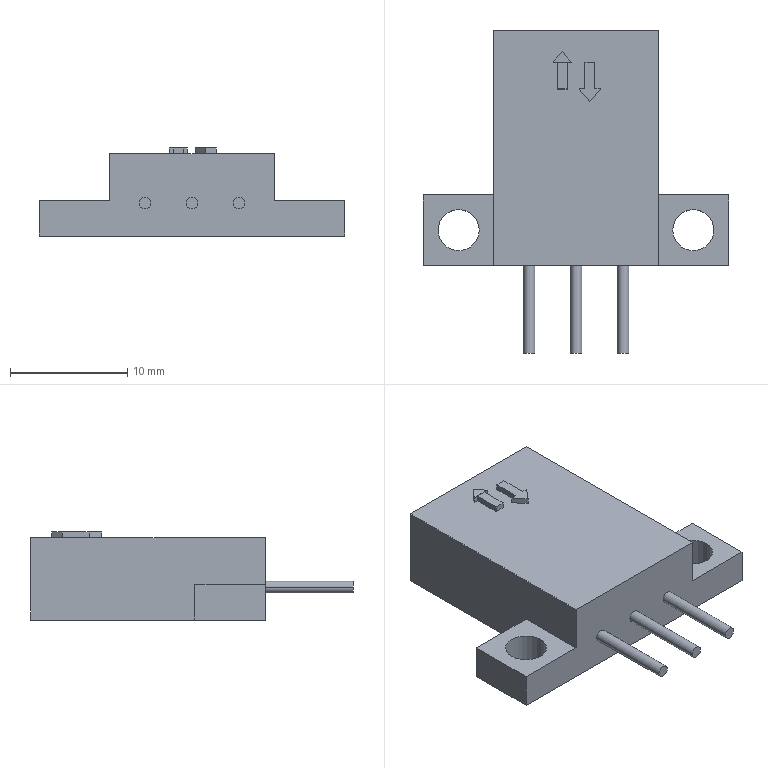Part | NX | features BREP 1 | 1 solid | 47 faces | box 26 x 27.5 x 7.5 mm | volume 2123 mm3 | plane 37 | cylinder 10 | commonest cylinder face diameters 1 x6 3.5 x4
STEP:
#1=CARTESIAN_POINT('',(4.,19.5,5.5));
#2=VERTEX_POINT('',#1);
#3=CARTESIAN_POINT('',(4.,19.5,1.5));
#4=VERTEX_POINT('',#3);
#5=CARTESIAN_POINT('',(4.,19.5,5.5));
#6=DIRECTION('',(0.,0.,-1.));
#7=VECTOR('',#6,1000.);
#8=LINE('',#5,#7);
#9=EDGE_CURVE('',#2,#4,#8,.T.);
#10=ORIENTED_EDGE('',*,*,#9,.T.);
#11=CARTESIAN_POINT('',(-4.,19.5,1.5));
#12=VERTEX_POINT('',#11);
#13=CARTESIAN_POINT('',(-4.,19.5,1.5));
#14=DIRECTION('',(-1.,0.,0.));
#15=VECTOR('',#14,1000.);
#16=LINE('',#13,#15);
#17=EDGE_CURVE('',#4,#12,#16,.T.);
#18=ORIENTED_EDGE('',*,*,#17,.T.);
#19=CARTESIAN_POINT('',(-4.,19.5,5.5));
#20=VERTEX_POINT('',#19);
#21=CARTESIAN_POINT('',(-4.,19.5,5.5));
#22=DIRECTION('',(0.,0.,1.));
#23=VECTOR('',#22,1000.);
#24=LINE('',#21,#23);
#25=EDGE_CURVE('',#12,#20,#24,.T.);
#26=ORIENTED_EDGE('',*,*,#25,.T.);
#27=CARTESIAN_POINT('',(-4.,19.5,5.5));
#28=DIRECTION('',(1.,0.,0.));
#29=VECTOR('',#28,1000.);
#30=LINE('',#27,#29);
#31=EDGE_CURVE('',#20,#2,#30,.T.);
#32=ORIENTED_EDGE('',*,*,#31,.T.);
#33=EDGE_LOOP('',(#10,#18,#26,#32));
#34=FACE_BOUND('',#33,.T.);
#35=CARTESIAN_POINT('',(0.,19.5,0.));
#36=DIRECTION('',(0.,-1.,0.));
#37=DIRECTION('',(0.,0.,-1.));
#38=AXIS2_PLACEMENT_3D('',#35,#36,#37);
#39=PLANE('',#38);
#40=ADVANCED_FACE('',(#34),#39,.F.);
#41=CARTESIAN_POINT('',(4.,20.,1.5));
#42=VERTEX_POINT('',#41);
#43=CARTESIAN_POINT('',(-4.,20.,1.5));
#44=VERTEX_POINT('',#43);
#45=CARTESIAN_POINT('',(-4.,20.,1.5));
#46=DIRECTION('',(-1.,0.,0.));
#47=VECTOR('',#46,1000.);
#48=LINE('',#45,#47);
#49=EDGE_CURVE('',#42,#44,#48,.T.);
#50=ORIENTED_EDGE('',*,*,#49,.T.);
#51=CARTESIAN_POINT('',(-4.,19.5,1.5));
#52=DIRECTION('',(0.,1.,0.));
#53=VECTOR('',#52,1000.);
#54=LINE('',#51,#53);
#55=EDGE_CURVE('',#12,#44,#54,.T.);
#56=ORIENTED_EDGE('',*,*,#55,.F.);
#57=ORIENTED_EDGE('',*,*,#17,.F.);
#58=CARTESIAN_POINT('',(4.,19.5,1.5));
#59=DIRECTION('',(0.,1.,0.));
#60=VECTOR('',#59,1000.);
#61=LINE('',#58,#60);
#62=EDGE_CURVE('',#4,#42,#61,.T.);
#63=ORIENTED_EDGE('',*,*,#62,.T.);
#64=EDGE_LOOP('',(#50,#56,#57,#63));
#65=FACE_BOUND('',#64,.T.);
#66=CARTESIAN_POINT('',(-4.,19.5,1.5));
#67=DIRECTION('',(0.,0.,-1.));
#68=DIRECTION('',(-1.,0.,0.));
#69=AXIS2_PLACEMENT_3D('',#66,#67,#68);
#70=PLANE('',#69);
#71=ADVANCED_FACE('',(#65),#70,.F.);
#72=CARTESIAN_POINT('',(-4.,20.,5.5));
#73=VERTEX_POINT('',#72);
#74=CARTESIAN_POINT('',(-4.,20.,5.5));
#75=DIRECTION('',(0.,0.,1.));
#76=VECTOR('',#75,1000.);
#77=LINE('',#74,#76);
#78=EDGE_CURVE('',#44,#73,#77,.T.);
#79=ORIENTED_EDGE('',*,*,#78,.T.);
#80=CARTESIAN_POINT('',(-4.,19.5,5.5));
#81=DIRECTION('',(0.,1.,0.));
#82=VECTOR('',#81,1000.);
#83=LINE('',#80,#82);
#84=EDGE_CURVE('',#20,#73,#83,.T.);
#85=ORIENTED_EDGE('',*,*,#84,.F.);
#86=ORIENTED_EDGE('',*,*,#25,.F.);
#87=ORIENTED_EDGE('',*,*,#55,.T.);
#88=EDGE_LOOP('',(#79,#85,#86,#87));
#89=FACE_BOUND('',#88,.T.);
#90=CARTESIAN_POINT('',(-4.,19.5,5.5));
#91=DIRECTION('',(-1.,0.,0.));
#92=DIRECTION('',(0.,0.,1.));
#93=AXIS2_PLACEMENT_3D('',#90,#91,#92);
#94=PLANE('',#93);
#95=ADVANCED_FACE('',(#89),#94,.F.);
#96=CARTESIAN_POINT('',(4.,20.,5.5));
#97=VERTEX_POINT('',#96);
#98=CARTESIAN_POINT('',(-4.,20.,5.5));
#99=DIRECTION('',(1.,0.,0.));
#100=VECTOR('',#99,1000.);
#101=LINE('',#98,#100);
#102=EDGE_CURVE('',#73,#97,#101,.T.);
#103=ORIENTED_EDGE('',*,*,#102,.T.);
#104=CARTESIAN_POINT('',(4.,19.5,5.5));
#105=DIRECTION('',(0.,1.,0.));
#106=VECTOR('',#105,1000.);
#107=LINE('',#104,#106);
#108=EDGE_CURVE('',#2,#97,#107,.T.);
#109=ORIENTED_EDGE('',*,*,#108,.F.);
#110=ORIENTED_EDGE('',*,*,#31,.F.);
#111=ORIENTED_EDGE('',*,*,#84,.T.);
#112=EDGE_LOOP('',(#103,#109,#110,#111));
#113=FACE_BOUND('',#112,.T.);
#114=CARTESIAN_POINT('',(-4.,19.5,5.5));
#115=DIRECTION('',(0.,0.,1.));
#116=DIRECTION('',(1.,0.,0.));
#117=AXIS2_PLACEMENT_3D('',#114,#115,#116);
#118=PLANE('',#117);
#119=ADVANCED_FACE('',(#113),#118,.F.);
#120=CARTESIAN_POINT('',(4.,20.,5.5));
#121=DIRECTION('',(0.,0.,-1.));
#122=VECTOR('',#121,1000.);
#123=LINE('',#120,#122);
#124=EDGE_CURVE('',#97,#42,#123,.T.);
#125=ORIENTED_EDGE('',*,*,#124,.T.);
#126=ORIENTED_EDGE('',*,*,#62,.F.);
#127=ORIENTED_EDGE('',*,*,#9,.F.);
#128=ORIENTED_EDGE('',*,*,#108,.T.);
#129=EDGE_LOOP('',(#125,#126,#127,#128));
#130=FACE_BOUND('',#129,.T.);
#131=CARTESIAN_POINT('',(4.,19.5,5.5));
#132=DIRECTION('',(1.,0.,0.));
#133=DIRECTION('',(0.,0.,-1.));
#134=AXIS2_PLACEMENT_3D('',#131,#132,#133);
#135=PLANE('',#134);
#136=ADVANCED_FACE('',(#130),#135,.F.);
#137=CARTESIAN_POINT('',(3.5,-7.5,2.8));
#138=VERTEX_POINT('',#137);
#139=CARTESIAN_POINT('',(4.5,-7.5,2.8));
#140=VERTEX_POINT('',#139);
#141=CARTESIAN_POINT('',(4.,-7.5,2.8));
#142=DIRECTION('',(0.,-1.,0.));
#143=DIRECTION('',(1.,0.,0.));
#144=AXIS2_PLACEMENT_3D('',#141,#142,#143);
#145=CIRCLE('',#144,0.5);
#146=EDGE_CURVE('',#138,#140,#145,.T.);
#147=ORIENTED_EDGE('',*,*,#146,.T.);
#148=CARTESIAN_POINT('',(4.,-7.5,2.8));
#149=DIRECTION('',(0.,-1.,0.));
#150=DIRECTION('',(1.,0.,0.));
#151=AXIS2_PLACEMENT_3D('',#148,#149,#150);
#152=CIRCLE('',#151,0.5);
#153=EDGE_CURVE('',#140,#138,#152,.T.);
#154=ORIENTED_EDGE('',*,*,#153,.T.);
#155=EDGE_LOOP('',(#147,#154));
#156=FACE_BOUND('',#155,.T.);
#157=CARTESIAN_POINT('',(4.,-7.5,2.8));
#158=DIRECTION('',(0.,-1.,0.));
#159=DIRECTION('',(1.,0.,0.));
#160=AXIS2_PLACEMENT_3D('',#157,#158,#159);
#161=PLANE('',#160);
#162=ADVANCED_FACE('',(#156),#161,.T.);
#163=CARTESIAN_POINT('',(4.5,0.,2.8));
#164=VERTEX_POINT('',#163);
#165=CARTESIAN_POINT('',(4.5,-7.5,2.8));
#166=DIRECTION('',(0.,1.,0.));
#167=VECTOR('',#166,1000.);
#168=LINE('',#165,#167);
#169=EDGE_CURVE('',#140,#164,#168,.T.);
#170=ORIENTED_EDGE('',*,*,#169,.F.);
#171=ORIENTED_EDGE('',*,*,#146,.F.);
#172=CARTESIAN_POINT('',(3.5,0.,2.8));
#173=VERTEX_POINT('',#172);
#174=CARTESIAN_POINT('',(3.5,-7.5,2.8));
#175=DIRECTION('',(0.,1.,0.));
#176=VECTOR('',#175,1000.);
#177=LINE('',#174,#176);
#178=EDGE_CURVE('',#138,#173,#177,.T.);
#179=ORIENTED_EDGE('',*,*,#178,.T.);
#180=CARTESIAN_POINT('',(4.,0.,2.8));
#181=DIRECTION('',(0.,-1.,0.));
#182=DIRECTION('',(-1.,0.,0.));
#183=AXIS2_PLACEMENT_3D('',#180,#181,#182);
#184=CIRCLE('',#183,0.5);
#185=EDGE_CURVE('',#173,#164,#184,.T.);
#186=ORIENTED_EDGE('',*,*,#185,.T.);
#187=EDGE_LOOP('',(#170,#171,#179,#186));
#188=FACE_BOUND('',#187,.T.);
#189=CARTESIAN_POINT('',(4.,-7.5,2.8));
#190=DIRECTION('',(0.,1.,0.));
#191=DIRECTION('',(-1.,0.,0.));
#192=AXIS2_PLACEMENT_3D('',#189,#190,#191);
#193=CYLINDRICAL_SURFACE('',#192,0.5);
#194=ADVANCED_FACE('',(#188),#193,.T.);
#195=CARTESIAN_POINT('',(-0.5,-7.5,2.8));
#196=VERTEX_POINT('',#195);
#197=CARTESIAN_POINT('',(0.5,-7.5,2.8));
#198=VERTEX_POINT('',#197);
#199=CARTESIAN_POINT('',(0.,-7.5,2.8));
#200=DIRECTION('',(0.,-1.,0.));
#201=DIRECTION('',(1.,0.,0.));
#202=AXIS2_PLACEMENT_3D('',#199,#200,#201);
#203=CIRCLE('',#202,0.5);
#204=EDGE_CURVE('',#196,#198,#203,.T.);
#205=ORIENTED_EDGE('',*,*,#204,.T.);
#206=CARTESIAN_POINT('',(0.,-7.5,2.8));
#207=DIRECTION('',(0.,-1.,0.));
#208=DIRECTION('',(1.,0.,0.));
#209=AXIS2_PLACEMENT_3D('',#206,#207,#208);
#210=CIRCLE('',#209,0.5);
#211=EDGE_CURVE('',#198,#196,#210,.T.);
#212=ORIENTED_EDGE('',*,*,#211,.T.);
#213=EDGE_LOOP('',(#205,#212));
#214=FACE_BOUND('',#213,.T.);
#215=CARTESIAN_POINT('',(0.,-7.5,2.8));
#216=DIRECTION('',(0.,-1.,0.));
#217=DIRECTION('',(1.,0.,0.));
#218=AXIS2_PLACEMENT_3D('',#215,#216,#217);
#219=PLANE('',#218);
#220=ADVANCED_FACE('',(#214),#219,.T.);
#221=CARTESIAN_POINT('',(0.5,0.,2.8));
#222=VERTEX_POINT('',#221);
#223=CARTESIAN_POINT('',(0.5,-7.5,2.8));
#224=DIRECTION('',(0.,1.,0.));
#225=VECTOR('',#224,1000.);
#226=LINE('',#223,#225);
#227=EDGE_CURVE('',#198,#222,#226,.T.);
#228=ORIENTED_EDGE('',*,*,#227,.F.);
#229=ORIENTED_EDGE('',*,*,#204,.F.);
#230=CARTESIAN_POINT('',(-0.5,0.,2.8));
#231=VERTEX_POINT('',#230);
#232=CARTESIAN_POINT('',(-0.5,-7.5,2.8));
#233=DIRECTION('',(0.,1.,0.));
#234=VECTOR('',#233,1000.);
#235=LINE('',#232,#234);
#236=EDGE_CURVE('',#196,#231,#235,.T.);
#237=ORIENTED_EDGE('',*,*,#236,.T.);
#238=CARTESIAN_POINT('',(0.,0.,2.8));
#239=DIRECTION('',(0.,-1.,0.));
#240=DIRECTION('',(-1.,0.,0.));
#241=AXIS2_PLACEMENT_3D('',#238,#239,#240);
#242=CIRCLE('',#241,0.5);
#243=EDGE_CURVE('',#231,#222,#242,.T.);
#244=ORIENTED_EDGE('',*,*,#243,.T.);
#245=EDGE_LOOP('',(#228,#229,#237,#244));
#246=FACE_BOUND('',#245,.T.);
#247=CARTESIAN_POINT('',(0.,-7.5,2.8));
#248=DIRECTION('',(0.,1.,0.));
#249=DIRECTION('',(-1.,0.,0.));
#250=AXIS2_PLACEMENT_3D('',#247,#248,#249);
#251=CYLINDRICAL_SURFACE('',#250,0.5);
#252=ADVANCED_FACE('',(#246),#251,.T.);
#253=CARTESIAN_POINT('',(-4.5,-7.5,2.8));
#254=VERTEX_POINT('',#253);
#255=CARTESIAN_POINT('',(-3.5,-7.5,2.8));
#256=VERTEX_POINT('',#255);
#257=CARTESIAN_POINT('',(-4.,-7.5,2.8));
#258=DIRECTION('',(0.,-1.,0.));
#259=DIRECTION('',(1.,0.,0.));
#260=AXIS2_PLACEMENT_3D('',#257,#258,#259);
#261=CIRCLE('',#260,0.5);
#262=EDGE_CURVE('',#254,#256,#261,.T.);
#263=ORIENTED_EDGE('',*,*,#262,.T.);
#264=CARTESIAN_POINT('',(-4.,-7.5,2.8));
#265=DIRECTION('',(0.,-1.,0.));
#266=DIRECTION('',(1.,0.,0.));
#267=AXIS2_PLACEMENT_3D('',#264,#265,#266);
#268=CIRCLE('',#267,0.5);
#269=EDGE_CURVE('',#256,#254,#268,.T.);
#270=ORIENTED_EDGE('',*,*,#269,.T.);
#271=EDGE_LOOP('',(#263,#270));
#272=FACE_BOUND('',#271,.T.);
#273=CARTESIAN_POINT('',(-4.,-7.5,2.8));
#274=DIRECTION('',(0.,-1.,0.));
#275=DIRECTION('',(1.,0.,0.));
#276=AXIS2_PLACEMENT_3D('',#273,#274,#275);
#277=PLANE('',#276);
#278=ADVANCED_FACE('',(#272),#277,.T.);
#279=CARTESIAN_POINT('',(-3.5,0.,2.8));
#280=VERTEX_POINT('',#279);
#281=CARTESIAN_POINT('',(-3.5,-7.5,2.8));
#282=DIRECTION('',(0.,1.,0.));
#283=VECTOR('',#282,1000.);
#284=LINE('',#281,#283);
#285=EDGE_CURVE('',#256,#280,#284,.T.);
#286=ORIENTED_EDGE('',*,*,#285,.F.);
#287=ORIENTED_EDGE('',*,*,#262,.F.);
#288=CARTESIAN_POINT('',(-4.5,0.,2.8));
#289=VERTEX_POINT('',#288);
#290=CARTESIAN_POINT('',(-4.5,-7.5,2.8));
#291=DIRECTION('',(0.,1.,0.));
#292=VECTOR('',#291,1000.);
#293=LINE('',#290,#292);
#294=EDGE_CURVE('',#254,#289,#293,.T.);
#295=ORIENTED_EDGE('',*,*,#294,.T.);
#296=CARTESIAN_POINT('',(-4.,0.,2.8));
#297=DIRECTION('',(0.,-1.,0.));
#298=DIRECTION('',(-1.,0.,0.));
#299=AXIS2_PLACEMENT_3D('',#296,#297,#298);
#300=CIRCLE('',#299,0.5);
#301=EDGE_CURVE('',#289,#280,#300,.T.);
#302=ORIENTED_EDGE('',*,*,#301,.T.);
#303=EDGE_LOOP('',(#286,#287,#295,#302));
#304=FACE_BOUND('',#303,.T.);
#305=CARTESIAN_POINT('',(-4.,-7.5,2.8));
#306=DIRECTION('',(0.,1.,0.));
#307=DIRECTION('',(-1.,0.,0.));
#308=AXIS2_PLACEMENT_3D('',#305,#306,#307);
#309=CYLINDRICAL_SURFACE('',#308,0.5);
#310=ADVANCED_FACE('',(#304),#309,.T.);
#311=CARTESIAN_POINT('',(-11.75,3.,3.));
#312=VERTEX_POINT('',#311);
#313=CARTESIAN_POINT('',(-11.75,3.,0.));
#314=VERTEX_POINT('',#313);
#315=CARTESIAN_POINT('',(-11.75,3.,3.));
#316=DIRECTION('',(0.,0.,1.));
#317=VECTOR('',#316,1000.);
#318=LINE('',#315,#317);
#319=EDGE_CURVE('',#312,#314,#318,.F.);
#320=ORIENTED_EDGE('',*,*,#319,.T.);
#321=CARTESIAN_POINT('',(-8.25,3.,0.));
#322=VERTEX_POINT('',#321);
#323=CARTESIAN_POINT('',(-10.,3.,0.));
#324=DIRECTION('',(0.,0.,1.));
#325=DIRECTION('',(1.,0.,0.));
#326=AXIS2_PLACEMENT_3D('',#323,#324,#325);
#327=CIRCLE('',#326,1.75);
#328=EDGE_CURVE('',#322,#314,#327,.T.);
#329=ORIENTED_EDGE('',*,*,#328,.F.);
#330=CARTESIAN_POINT('',(-8.25,3.,3.));
#331=VERTEX_POINT('',#330);
#332=CARTESIAN_POINT('',(-8.25,3.,3.));
#333=DIRECTION('',(0.,0.,1.));
#334=VECTOR('',#333,1000.);
#335=LINE('',#332,#334);
#336=EDGE_CURVE('',#331,#322,#335,.F.);
#337=ORIENTED_EDGE('',*,*,#336,.F.);
#338=CARTESIAN_POINT('',(-10.,3.,3.));
#339=DIRECTION('',(0.,0.,1.));
#340=DIRECTION('',(1.,0.,0.));
#341=AXIS2_PLACEMENT_3D('',#338,#339,#340);
#342=CIRCLE('',#341,1.75);
#343=EDGE_CURVE('',#331,#312,#342,.T.);
#344=ORIENTED_EDGE('',*,*,#343,.T.);
#345=EDGE_LOOP('',(#320,#329,#337,#344));
#346=FACE_BOUND('',#345,.T.);
#347=CARTESIAN_POINT('',(-10.,3.,3.));
#348=DIRECTION('',(0.,0.,1.));
#349=DIRECTION('',(1.,0.,0.));
#350=AXIS2_PLACEMENT_3D('',#347,#348,#349);
#351=CYLINDRICAL_SURFACE('',#350,1.75);
#352=ADVANCED_FACE('',(#346),#351,.F.);
#353=CARTESIAN_POINT('',(8.25,3.,3.));
#354=VERTEX_POINT('',#353);
#355=CARTESIAN_POINT('',(8.25,3.,0.));
#356=VERTEX_POINT('',#355);
#357=CARTESIAN_POINT('',(8.25,3.,3.));
#358=DIRECTION('',(0.,0.,1.));
#359=VECTOR('',#358,1000.);
#360=LINE('',#357,#359);
#361=EDGE_CURVE('',#354,#356,#360,.F.);
#362=ORIENTED_EDGE('',*,*,#361,.T.);
#363=CARTESIAN_POINT('',(11.75,3.,0.));
#364=VERTEX_POINT('',#363);
#365=CARTESIAN_POINT('',(10.,3.,0.));
#366=DIRECTION('',(0.,0.,1.));
#367=DIRECTION('',(1.,0.,0.));
#368=AXIS2_PLACEMENT_3D('',#365,#366,#367);
#369=CIRCLE('',#368,1.75);
#370=EDGE_CURVE('',#364,#356,#369,.T.);
#371=ORIENTED_EDGE('',*,*,#370,.F.);
#372=CARTESIAN_POINT('',(11.75,3.,3.));
#373=VERTEX_POINT('',#372);
#374=CARTESIAN_POINT('',(11.75,3.,3.));
#375=DIRECTION('',(0.,0.,1.));
#376=VECTOR('',#375,1000.);
#377=LINE('',#374,#376);
#378=EDGE_CURVE('',#373,#364,#377,.F.);
#379=ORIENTED_EDGE('',*,*,#378,.F.);
#380=CARTESIAN_POINT('',(10.,3.,3.));
#381=DIRECTION('',(0.,0.,1.));
#382=DIRECTION('',(1.,0.,0.));
#383=AXIS2_PLACEMENT_3D('',#380,#381,#382);
#384=CIRCLE('',#383,1.75);
#385=EDGE_CURVE('',#373,#354,#384,.T.);
#386=ORIENTED_EDGE('',*,*,#385,.T.);
#387=EDGE_LOOP('',(#362,#371,#379,#386));
#388=FACE_BOUND('',#387,.T.);
#389=CARTESIAN_POINT('',(10.,3.,3.));
#390=DIRECTION('',(0.,0.,1.));
#391=DIRECTION('',(1.,0.,0.));
#392=AXIS2_PLACEMENT_3D('',#389,#390,#391);
#393=CYLINDRICAL_SURFACE('',#392,1.75);
#394=ADVANCED_FACE('',(#388),#393,.F.);
#395=CARTESIAN_POINT('',(1.592,17.295,7.5));
#396=VERTEX_POINT('',#395);
#397=CARTESIAN_POINT('',(1.592,15.02,7.5));
#398=VERTEX_POINT('',#397);
#399=CARTESIAN_POINT('',(1.592,0.,7.5));
#400=DIRECTION('',(0.,-1.,0.));
#401=VECTOR('',#400,1000.);
#402=LINE('',#399,#401);
#403=EDGE_CURVE('',#396,#398,#402,.T.);
#404=ORIENTED_EDGE('',*,*,#403,.F.);
#405=CARTESIAN_POINT('',(0.7557,17.295,7.5));
#406=VERTEX_POINT('',#405);
#407=CARTESIAN_POINT('',(0.,17.295,7.5));
#408=DIRECTION('',(1.,0.,0.));
#409=VECTOR('',#408,1000.);
#410=LINE('',#407,#409);
#411=EDGE_CURVE('',#406,#396,#410,.T.);
#412=ORIENTED_EDGE('',*,*,#411,.F.);
#413=CARTESIAN_POINT('',(0.7557,15.02,7.5));
#414=VERTEX_POINT('',#413);
#415=CARTESIAN_POINT('',(0.7557,0.,7.5));
#416=DIRECTION('',(0.,-1.,0.));
#417=VECTOR('',#416,1000.);
#418=LINE('',#415,#417);
#419=EDGE_CURVE('',#406,#414,#418,.T.);
#420=ORIENTED_EDGE('',*,*,#419,.T.);
#421=CARTESIAN_POINT('',(0.2749,15.02,7.5));
#422=VERTEX_POINT('',#421);
#423=CARTESIAN_POINT('',(0.,15.02,7.5));
#424=DIRECTION('',(1.,0.,0.));
#425=VECTOR('',#424,1000.);
#426=LINE('',#423,#425);
#427=EDGE_CURVE('',#422,#414,#426,.T.);
#428=ORIENTED_EDGE('',*,*,#427,.F.);
#429=CARTESIAN_POINT('',(1.174,13.95,7.5));
#430=VERTEX_POINT('',#429);
#431=CARTESIAN_POINT('',(7.559,6.351,7.5));
#432=DIRECTION('',(-0.6433,0.7656,0.));
#433=VECTOR('',#432,1000.);
#434=LINE('',#431,#433);
#435=EDGE_CURVE('',#430,#422,#434,.T.);
#436=ORIENTED_EDGE('',*,*,#435,.F.);
#437=CARTESIAN_POINT('',(2.073,15.02,7.5));
#438=VERTEX_POINT('',#437);
#439=CARTESIAN_POINT('',(-6.183,5.195,7.5));
#440=DIRECTION('',(-0.6433,-0.7656,0.));
#441=VECTOR('',#440,1000.);
#442=LINE('',#439,#441);
#443=EDGE_CURVE('',#438,#430,#442,.T.);
#444=ORIENTED_EDGE('',*,*,#443,.F.);
#445=CARTESIAN_POINT('',(0.,15.02,7.5));
#446=DIRECTION('',(1.,0.,0.));
#447=VECTOR('',#446,1000.);
#448=LINE('',#445,#447);
#449=EDGE_CURVE('',#398,#438,#448,.T.);
#450=ORIENTED_EDGE('',*,*,#449,.F.);
#451=EDGE_LOOP('',(#404,#412,#420,#428,#436,#444,#450));
#452=FACE_BOUND('',#451,.T.);
#453=CARTESIAN_POINT('',(0.,0.,7.5));
#454=DIRECTION('',(0.,0.,1.));
#455=DIRECTION('',(1.,0.,0.));
#456=AXIS2_PLACEMENT_3D('',#453,#454,#455);
#457=PLANE('',#456);
#458=ADVANCED_FACE('',(#452),#457,.T.);
#459=CARTESIAN_POINT('',(1.592,15.02,7.));
#460=VERTEX_POINT('',#459);
#461=CARTESIAN_POINT('',(2.073,15.02,7.));
#462=VERTEX_POINT('',#461);
#463=CARTESIAN_POINT('',(0.,15.02,7.));
#464=DIRECTION('',(1.,0.,0.));
#465=VECTOR('',#464,1000.);
#466=LINE('',#463,#465);
#467=EDGE_CURVE('',#460,#462,#466,.T.);
#468=ORIENTED_EDGE('',*,*,#467,.F.);
#469=CARTESIAN_POINT('',(1.592,15.02,7.5));
#470=DIRECTION('',(0.,0.,-1.));
#471=VECTOR('',#470,1000.);
#472=LINE('',#469,#471);
#473=EDGE_CURVE('',#398,#460,#472,.T.);
#474=ORIENTED_EDGE('',*,*,#473,.F.);
#475=ORIENTED_EDGE('',*,*,#449,.T.);
#476=CARTESIAN_POINT('',(2.073,15.02,7.5));
#477=DIRECTION('',(0.,0.,-1.));
#478=VECTOR('',#477,1000.);
#479=LINE('',#476,#478);
#480=EDGE_CURVE('',#438,#462,#479,.T.);
#481=ORIENTED_EDGE('',*,*,#480,.T.);
#482=EDGE_LOOP('',(#468,#474,#475,#481));
#483=FACE_BOUND('',#482,.T.);
#484=CARTESIAN_POINT('',(0.,15.02,7.5));
#485=DIRECTION('',(0.,1.,0.));
#486=DIRECTION('',(0.,0.,1.));
#487=AXIS2_PLACEMENT_3D('',#484,#485,#486);
#488=PLANE('',#487);
#489=ADVANCED_FACE('',(#483),#488,.T.);
#490=CARTESIAN_POINT('',(1.174,13.95,7.));
#491=VERTEX_POINT('',#490);
#492=CARTESIAN_POINT('',(-6.183,5.195,7.));
#493=DIRECTION('',(-0.6433,-0.7656,0.));
#494=VECTOR('',#493,1000.);
#495=LINE('',#492,#494);
#496=EDGE_CURVE('',#462,#491,#495,.T.);
#497=ORIENTED_EDGE('',*,*,#496,.F.);
#498=ORIENTED_EDGE('',*,*,#480,.F.);
#499=ORIENTED_EDGE('',*,*,#443,.T.);
#500=CARTESIAN_POINT('',(1.174,13.95,7.5));
#501=DIRECTION('',(0.,0.,-1.));
#502=VECTOR('',#501,1000.);
#503=LINE('',#500,#502);
#504=EDGE_CURVE('',#430,#491,#503,.T.);
#505=ORIENTED_EDGE('',*,*,#504,.T.);
#506=EDGE_LOOP('',(#497,#498,#499,#505));
#507=FACE_BOUND('',#506,.T.);
#508=CARTESIAN_POINT('',(-6.183,5.195,7.5));
#509=DIRECTION('',(0.7656,-0.6433,0.));
#510=DIRECTION('',(0.6433,0.7656,0.));
#511=AXIS2_PLACEMENT_3D('',#508,#509,#510);
#512=PLANE('',#511);
#513=ADVANCED_FACE('',(#507),#512,.T.);
#514=CARTESIAN_POINT('',(0.2749,15.02,7.));
#515=VERTEX_POINT('',#514);
#516=CARTESIAN_POINT('',(7.559,6.351,7.));
#517=DIRECTION('',(-0.6433,0.7656,0.));
#518=VECTOR('',#517,1000.);
#519=LINE('',#516,#518);
#520=EDGE_CURVE('',#491,#515,#519,.T.);
#521=ORIENTED_EDGE('',*,*,#520,.F.);
#522=ORIENTED_EDGE('',*,*,#504,.F.);
#523=ORIENTED_EDGE('',*,*,#435,.T.);
#524=CARTESIAN_POINT('',(0.2749,15.02,7.5));
#525=DIRECTION('',(0.,0.,-1.));
#526=VECTOR('',#525,1000.);
#527=LINE('',#524,#526);
#528=EDGE_CURVE('',#422,#515,#527,.T.);
#529=ORIENTED_EDGE('',*,*,#528,.T.);
#530=EDGE_LOOP('',(#521,#522,#523,#529));
#531=FACE_BOUND('',#530,.T.);
#532=CARTESIAN_POINT('',(7.559,6.351,7.5));
#533=DIRECTION('',(-0.7656,-0.6433,0.));
#534=DIRECTION('',(0.6433,-0.7656,0.));
#535=AXIS2_PLACEMENT_3D('',#532,#533,#534);
#536=PLANE('',#535);
#537=ADVANCED_FACE('',(#531),#536,.T.);
#538=CARTESIAN_POINT('',(0.7557,15.02,7.));
#539=VERTEX_POINT('',#538);
#540=CARTESIAN_POINT('',(0.,15.02,7.));
#541=DIRECTION('',(1.,0.,0.));
#542=VECTOR('',#541,1000.);
#543=LINE('',#540,#542);
#544=EDGE_CURVE('',#515,#539,#543,.T.);
#545=ORIENTED_EDGE('',*,*,#544,.F.);
#546=ORIENTED_EDGE('',*,*,#528,.F.);
#547=ORIENTED_EDGE('',*,*,#427,.T.);
#548=CARTESIAN_POINT('',(0.7557,15.02,7.5));
#549=DIRECTION('',(0.,0.,-1.));
#550=VECTOR('',#549,1000.);
#551=LINE('',#548,#550);
#552=EDGE_CURVE('',#414,#539,#551,.T.);
#553=ORIENTED_EDGE('',*,*,#552,.T.);
#554=EDGE_LOOP('',(#545,#546,#547,#553));
#555=FACE_BOUND('',#554,.T.);
#556=CARTESIAN_POINT('',(0.,15.02,7.5));
#557=DIRECTION('',(0.,1.,0.));
#558=DIRECTION('',(0.,0.,1.));
#559=AXIS2_PLACEMENT_3D('',#556,#557,#558);
#560=PLANE('',#559);
#561=ADVANCED_FACE('',(#555),#560,.T.);
#562=CARTESIAN_POINT('',(0.7557,17.295,7.));
#563=VERTEX_POINT('',#562);
#564=CARTESIAN_POINT('',(0.7557,0.,7.));
#565=DIRECTION('',(0.,-1.,0.));
#566=VECTOR('',#565,1000.);
#567=LINE('',#564,#566);
#568=EDGE_CURVE('',#563,#539,#567,.T.);
#569=ORIENTED_EDGE('',*,*,#568,.T.);
#570=ORIENTED_EDGE('',*,*,#552,.F.);
#571=ORIENTED_EDGE('',*,*,#419,.F.);
#572=CARTESIAN_POINT('',(0.7557,17.295,7.5));
#573=DIRECTION('',(0.,0.,-1.));
#574=VECTOR('',#573,1000.);
#575=LINE('',#572,#574);
#576=EDGE_CURVE('',#406,#563,#575,.T.);
#577=ORIENTED_EDGE('',*,*,#576,.T.);
#578=EDGE_LOOP('',(#569,#570,#571,#577));
#579=FACE_BOUND('',#578,.T.);
#580=CARTESIAN_POINT('',(0.7557,0.,7.5));
#581=DIRECTION('',(1.,0.,0.));
#582=DIRECTION('',(0.,1.,0.));
#583=AXIS2_PLACEMENT_3D('',#580,#581,#582);
#584=PLANE('',#583);
#585=ADVANCED_FACE('',(#579),#584,.F.);
#586=CARTESIAN_POINT('',(1.592,17.295,7.));
#587=VERTEX_POINT('',#586);
#588=CARTESIAN_POINT('',(0.,17.295,7.));
#589=DIRECTION('',(1.,0.,0.));
#590=VECTOR('',#589,1000.);
#591=LINE('',#588,#590);
#592=EDGE_CURVE('',#563,#587,#591,.T.);
#593=ORIENTED_EDGE('',*,*,#592,.F.);
#594=ORIENTED_EDGE('',*,*,#576,.F.);
#595=ORIENTED_EDGE('',*,*,#411,.T.);
#596=CARTESIAN_POINT('',(1.592,17.295,7.5));
#597=DIRECTION('',(0.,0.,-1.));
#598=VECTOR('',#597,1000.);
#599=LINE('',#596,#598);
#600=EDGE_CURVE('',#396,#587,#599,.T.);
#601=ORIENTED_EDGE('',*,*,#600,.T.);
#602=EDGE_LOOP('',(#593,#594,#595,#601));
#603=FACE_BOUND('',#602,.T.);
#604=CARTESIAN_POINT('',(0.,17.295,7.5));
#605=DIRECTION('',(0.,1.,0.));
#606=DIRECTION('',(-1.,0.,0.));
#607=AXIS2_PLACEMENT_3D('',#604,#605,#606);
#608=PLANE('',#607);
#609=ADVANCED_FACE('',(#603),#608,.T.);
#610=CARTESIAN_POINT('',(1.592,0.,7.));
#611=DIRECTION('',(0.,-1.,0.));
#612=VECTOR('',#611,1000.);
#613=LINE('',#610,#612);
#614=EDGE_CURVE('',#587,#460,#613,.T.);
#615=ORIENTED_EDGE('',*,*,#614,.F.);
#616=ORIENTED_EDGE('',*,*,#600,.F.);
#617=ORIENTED_EDGE('',*,*,#403,.T.);
#618=ORIENTED_EDGE('',*,*,#473,.T.);
#619=EDGE_LOOP('',(#615,#616,#617,#618));
#620=FACE_BOUND('',#619,.T.);
#621=CARTESIAN_POINT('',(1.592,0.,7.5));
#622=DIRECTION('',(1.,0.,0.));
#623=DIRECTION('',(0.,0.,-1.));
#624=AXIS2_PLACEMENT_3D('',#621,#622,#623);
#625=PLANE('',#624);
#626=ADVANCED_FACE('',(#620),#625,.T.);
#627=CARTESIAN_POINT('',(-1.592,15.02,7.5));
#628=VERTEX_POINT('',#627);
#629=CARTESIAN_POINT('',(-0.7557,15.02,7.5));
#630=VERTEX_POINT('',#629);
#631=CARTESIAN_POINT('',(0.,15.02,7.5));
#632=DIRECTION('',(1.,0.,0.));
#633=VECTOR('',#632,1000.);
#634=LINE('',#631,#633);
#635=EDGE_CURVE('',#628,#630,#634,.T.);
#636=ORIENTED_EDGE('',*,*,#635,.T.);
#637=CARTESIAN_POINT('',(-0.7557,17.295,7.5));
#638=VERTEX_POINT('',#637);
#639=CARTESIAN_POINT('',(-0.7557,0.,7.5));
#640=DIRECTION('',(0.,1.,0.));
#641=VECTOR('',#640,1000.);
#642=LINE('',#639,#641);
#643=EDGE_CURVE('',#630,#638,#642,.T.);
#644=ORIENTED_EDGE('',*,*,#643,.T.);
#645=CARTESIAN_POINT('',(-1.592,17.295,7.5));
#646=VERTEX_POINT('',#645);
#647=CARTESIAN_POINT('',(0.,17.295,7.5));
#648=DIRECTION('',(1.,0.,0.));
#649=VECTOR('',#648,1000.);
#650=LINE('',#647,#649);
#651=EDGE_CURVE('',#646,#638,#650,.T.);
#652=ORIENTED_EDGE('',*,*,#651,.F.);
#653=CARTESIAN_POINT('',(-1.592,0.,7.5));
#654=DIRECTION('',(0.,1.,0.));
#655=VECTOR('',#654,1000.);
#656=LINE('',#653,#655);
#657=EDGE_CURVE('',#628,#646,#656,.T.);
#658=ORIENTED_EDGE('',*,*,#657,.F.);
#659=EDGE_LOOP('',(#636,#644,#652,#658));
#660=FACE_BOUND('',#659,.T.);
#661=CARTESIAN_POINT('',(0.,0.,7.5));
#662=DIRECTION('',(0.,0.,1.));
#663=DIRECTION('',(1.,0.,0.));
#664=AXIS2_PLACEMENT_3D('',#661,#662,#663);
#665=PLANE('',#664);
#666=ADVANCED_FACE('',(#660),#665,.T.);
#667=CARTESIAN_POINT('',(-1.592,15.02,7.));
#668=VERTEX_POINT('',#667);
#669=CARTESIAN_POINT('',(-1.592,17.295,7.));
#670=VERTEX_POINT('',#669);
#671=CARTESIAN_POINT('',(-1.592,0.,7.));
#672=DIRECTION('',(0.,1.,0.));
#673=VECTOR('',#672,1000.);
#674=LINE('',#671,#673);
#675=EDGE_CURVE('',#668,#670,#674,.T.);
#676=ORIENTED_EDGE('',*,*,#675,.F.);
#677=CARTESIAN_POINT('',(-1.592,15.02,7.5));
#678=DIRECTION('',(0.,0.,-1.));
#679=VECTOR('',#678,1000.);
#680=LINE('',#677,#679);
#681=EDGE_CURVE('',#628,#668,#680,.T.);
#682=ORIENTED_EDGE('',*,*,#681,.F.);
#683=ORIENTED_EDGE('',*,*,#657,.T.);
#684=CARTESIAN_POINT('',(-1.592,17.295,7.5));
#685=DIRECTION('',(0.,0.,-1.));
#686=VECTOR('',#685,1000.);
#687=LINE('',#684,#686);
#688=EDGE_CURVE('',#646,#670,#687,.T.);
#689=ORIENTED_EDGE('',*,*,#688,.T.);
#690=EDGE_LOOP('',(#676,#682,#683,#689));
#691=FACE_BOUND('',#690,.T.);
#692=CARTESIAN_POINT('',(-1.592,0.,7.5));
#693=DIRECTION('',(-1.,0.,0.));
#694=DIRECTION('',(0.,0.,1.));
#695=AXIS2_PLACEMENT_3D('',#692,#693,#694);
#696=PLANE('',#695);
#697=ADVANCED_FACE('',(#691),#696,.T.);
#698=CARTESIAN_POINT('',(-0.7557,17.295,7.));
#699=VERTEX_POINT('',#698);
#700=CARTESIAN_POINT('',(0.,17.295,7.));
#701=DIRECTION('',(1.,0.,0.));
#702=VECTOR('',#701,1000.);
#703=LINE('',#700,#702);
#704=EDGE_CURVE('',#670,#699,#703,.T.);
#705=ORIENTED_EDGE('',*,*,#704,.F.);
#706=ORIENTED_EDGE('',*,*,#688,.F.);
#707=ORIENTED_EDGE('',*,*,#651,.T.);
#708=CARTESIAN_POINT('',(-0.7557,17.295,7.5));
#709=DIRECTION('',(0.,0.,-1.));
#710=VECTOR('',#709,1000.);
#711=LINE('',#708,#710);
#712=EDGE_CURVE('',#638,#699,#711,.T.);
#713=ORIENTED_EDGE('',*,*,#712,.T.);
#714=EDGE_LOOP('',(#705,#706,#707,#713));
#715=FACE_BOUND('',#714,.T.);
#716=CARTESIAN_POINT('',(0.,17.295,7.5));
#717=DIRECTION('',(0.,1.,0.));
#718=DIRECTION('',(0.,0.,1.));
#719=AXIS2_PLACEMENT_3D('',#716,#717,#718);
#720=PLANE('',#719);
#721=ADVANCED_FACE('',(#715),#720,.T.);
#722=CARTESIAN_POINT('',(-0.7557,15.02,7.));
#723=VERTEX_POINT('',#722);
#724=CARTESIAN_POINT('',(-0.7557,0.,7.));
#725=DIRECTION('',(0.,1.,0.));
#726=VECTOR('',#725,1000.);
#727=LINE('',#724,#726);
#728=EDGE_CURVE('',#723,#699,#727,.T.);
#729=ORIENTED_EDGE('',*,*,#728,.T.);
#730=ORIENTED_EDGE('',*,*,#712,.F.);
#731=ORIENTED_EDGE('',*,*,#643,.F.);
#732=CARTESIAN_POINT('',(-0.7557,15.02,7.5));
#733=DIRECTION('',(0.,0.,-1.));
#734=VECTOR('',#733,1000.);
#735=LINE('',#732,#734);
#736=EDGE_CURVE('',#630,#723,#735,.T.);
#737=ORIENTED_EDGE('',*,*,#736,.T.);
#738=EDGE_LOOP('',(#729,#730,#731,#737));
#739=FACE_BOUND('',#738,.T.);
#740=CARTESIAN_POINT('',(-0.7557,0.,7.5));
#741=DIRECTION('',(-1.,0.,0.));
#742=DIRECTION('',(0.,-1.,0.));
#743=AXIS2_PLACEMENT_3D('',#740,#741,#742);
#744=PLANE('',#743);
#745=ADVANCED_FACE('',(#739),#744,.F.);
#746=CARTESIAN_POINT('',(0.,15.02,7.));
#747=DIRECTION('',(1.,0.,0.));
#748=VECTOR('',#747,1000.);
#749=LINE('',#746,#748);
#750=EDGE_CURVE('',#668,#723,#749,.T.);
#751=ORIENTED_EDGE('',*,*,#750,.T.);
#752=ORIENTED_EDGE('',*,*,#736,.F.);
#753=ORIENTED_EDGE('',*,*,#635,.F.);
#754=ORIENTED_EDGE('',*,*,#681,.T.);
#755=EDGE_LOOP('',(#751,#752,#753,#754));
#756=FACE_BOUND('',#755,.T.);
#757=CARTESIAN_POINT('',(0.,15.02,7.5));
#758=DIRECTION('',(0.,1.,0.));
#759=DIRECTION('',(0.,0.,1.));
#760=AXIS2_PLACEMENT_3D('',#757,#758,#759);
#761=PLANE('',#760);
#762=ADVANCED_FACE('',(#756),#761,.F.);
#763=CARTESIAN_POINT('',(-0.3905,17.301,7.5));
#764=VERTEX_POINT('',#763);
#765=CARTESIAN_POINT('',(-1.957,17.301,7.5));
#766=VERTEX_POINT('',#765);
#767=CARTESIAN_POINT('',(0.,17.301,7.5));
#768=DIRECTION('',(-1.,0.,0.));
#769=VECTOR('',#768,1000.);
#770=LINE('',#767,#769);
#771=EDGE_CURVE('',#764,#766,#770,.T.);
#772=ORIENTED_EDGE('',*,*,#771,.F.);
#773=CARTESIAN_POINT('',(-1.174,18.21,7.5));
#774=VERTEX_POINT('',#773);
#775=CARTESIAN_POINT('',(8.333,7.186,7.5));
#776=DIRECTION('',(0.6531,-0.7573,0.));
#777=VECTOR('',#776,1000.);
#778=LINE('',#775,#777);
#779=EDGE_CURVE('',#774,#764,#778,.T.);
#780=ORIENTED_EDGE('',*,*,#779,.F.);
#781=CARTESIAN_POINT('',(-9.679,8.347,7.5));
#782=DIRECTION('',(0.6531,0.7573,0.));
#783=VECTOR('',#782,1000.);
#784=LINE('',#781,#783);
#785=EDGE_CURVE('',#766,#774,#784,.T.);
#786=ORIENTED_EDGE('',*,*,#785,.F.);
#787=EDGE_LOOP('',(#772,#780,#786));
#788=FACE_BOUND('',#787,.T.);
#789=CARTESIAN_POINT('',(0.,0.,7.5));
#790=DIRECTION('',(0.,0.,1.));
#791=DIRECTION('',(1.,0.,0.));
#792=AXIS2_PLACEMENT_3D('',#789,#790,#791);
#793=PLANE('',#792);
#794=ADVANCED_FACE('',(#788),#793,.T.);
#795=CARTESIAN_POINT('',(-1.957,17.301,7.));
#796=VERTEX_POINT('',#795);
#797=CARTESIAN_POINT('',(-1.174,18.21,7.));
#798=VERTEX_POINT('',#797);
#799=CARTESIAN_POINT('',(-9.679,8.347,7.));
#800=DIRECTION('',(0.6531,0.7573,0.));
#801=VECTOR('',#800,1000.);
#802=LINE('',#799,#801);
#803=EDGE_CURVE('',#796,#798,#802,.T.);
#804=ORIENTED_EDGE('',*,*,#803,.F.);
#805=CARTESIAN_POINT('',(-1.957,17.301,7.5));
#806=DIRECTION('',(0.,0.,-1.));
#807=VECTOR('',#806,1000.);
#808=LINE('',#805,#807);
#809=EDGE_CURVE('',#766,#796,#808,.T.);
#810=ORIENTED_EDGE('',*,*,#809,.F.);
#811=ORIENTED_EDGE('',*,*,#785,.T.);
#812=CARTESIAN_POINT('',(-1.174,18.21,7.5));
#813=DIRECTION('',(0.,0.,-1.));
#814=VECTOR('',#813,1000.);
#815=LINE('',#812,#814);
#816=EDGE_CURVE('',#774,#798,#815,.T.);
#817=ORIENTED_EDGE('',*,*,#816,.T.);
#818=EDGE_LOOP('',(#804,#810,#811,#817));
#819=FACE_BOUND('',#818,.T.);
#820=CARTESIAN_POINT('',(-9.679,8.347,7.5));
#821=DIRECTION('',(-0.7573,0.6531,0.));
#822=DIRECTION('',(-0.6531,-0.7573,0.));
#823=AXIS2_PLACEMENT_3D('',#820,#821,#822);
#824=PLANE('',#823);
#825=ADVANCED_FACE('',(#819),#824,.T.);
#826=CARTESIAN_POINT('',(-0.3905,17.301,7.));
#827=VERTEX_POINT('',#826);
#828=CARTESIAN_POINT('',(8.333,7.186,7.));
#829=DIRECTION('',(0.6531,-0.7573,0.));
#830=VECTOR('',#829,1000.);
#831=LINE('',#828,#830);
#832=EDGE_CURVE('',#798,#827,#831,.T.);
#833=ORIENTED_EDGE('',*,*,#832,.F.);
#834=ORIENTED_EDGE('',*,*,#816,.F.);
#835=ORIENTED_EDGE('',*,*,#779,.T.);
#836=CARTESIAN_POINT('',(-0.3905,17.301,7.5));
#837=DIRECTION('',(0.,0.,-1.));
#838=VECTOR('',#837,1000.);
#839=LINE('',#836,#838);
#840=EDGE_CURVE('',#764,#827,#839,.T.);
#841=ORIENTED_EDGE('',*,*,#840,.T.);
#842=EDGE_LOOP('',(#833,#834,#835,#841));
#843=FACE_BOUND('',#842,.T.);
#844=CARTESIAN_POINT('',(8.333,7.186,7.5));
#845=DIRECTION('',(0.7573,0.6531,0.));
#846=DIRECTION('',(-0.6531,0.7573,0.));
#847=AXIS2_PLACEMENT_3D('',#844,#845,#846);
#848=PLANE('',#847);
#849=ADVANCED_FACE('',(#843),#848,.T.);
#850=CARTESIAN_POINT('',(0.,17.301,7.));
#851=DIRECTION('',(-1.,0.,0.));
#852=VECTOR('',#851,1000.);
#853=LINE('',#850,#852);
#854=EDGE_CURVE('',#827,#796,#853,.T.);
#855=ORIENTED_EDGE('',*,*,#854,.F.);
#856=ORIENTED_EDGE('',*,*,#840,.F.);
#857=ORIENTED_EDGE('',*,*,#771,.T.);
#858=ORIENTED_EDGE('',*,*,#809,.T.);
#859=EDGE_LOOP('',(#855,#856,#857,#858));
#860=FACE_BOUND('',#859,.T.);
#861=CARTESIAN_POINT('',(0.,17.301,7.5));
#862=DIRECTION('',(0.,-1.,0.));
#863=DIRECTION('',(0.,0.,-1.));
#864=AXIS2_PLACEMENT_3D('',#861,#862,#863);
#865=PLANE('',#864);
#866=ADVANCED_FACE('',(#860),#865,.T.);
#867=CARTESIAN_POINT('',(13.,6.,3.));
#868=VERTEX_POINT('',#867);
#869=CARTESIAN_POINT('',(13.,0.,3.));
#870=VERTEX_POINT('',#869);
#871=CARTESIAN_POINT('',(13.,6.,3.));
#872=DIRECTION('',(0.,-1.,0.));
#873=VECTOR('',#872,1000.);
#874=LINE('',#871,#873);
#875=EDGE_CURVE('',#868,#870,#874,.T.);
#876=ORIENTED_EDGE('',*,*,#875,.F.);
#877=CARTESIAN_POINT('',(7.,6.,3.));
#878=VERTEX_POINT('',#877);
#879=CARTESIAN_POINT('',(13.,6.,3.));
#880=DIRECTION('',(1.,0.,0.));
#881=VECTOR('',#880,1000.);
#882=LINE('',#879,#881);
#883=EDGE_CURVE('',#878,#868,#882,.T.);
#884=ORIENTED_EDGE('',*,*,#883,.F.);
#885=CARTESIAN_POINT('',(7.,0.,3.));
#886=VERTEX_POINT('',#885);
#887=CARTESIAN_POINT('',(7.,6.,3.));
#888=DIRECTION('',(0.,1.,0.));
#889=VECTOR('',#888,1000.);
#890=LINE('',#887,#889);
#891=EDGE_CURVE('',#886,#878,#890,.T.);
#892=ORIENTED_EDGE('',*,*,#891,.F.);
#893=CARTESIAN_POINT('',(13.,0.,3.));
#894=DIRECTION('',(-1.,0.,0.));
#895=VECTOR('',#894,1000.);
#896=LINE('',#893,#895);
#897=EDGE_CURVE('',#870,#886,#896,.T.);
#898=ORIENTED_EDGE('',*,*,#897,.F.);
#899=EDGE_LOOP('',(#876,#884,#892,#898));
#900=FACE_BOUND('',#899,.T.);
#901=ORIENTED_EDGE('',*,*,#385,.F.);
#902=CARTESIAN_POINT('',(10.,3.,3.));
#903=DIRECTION('',(0.,0.,1.));
#904=DIRECTION('',(1.,0.,0.));
#905=AXIS2_PLACEMENT_3D('',#902,#903,#904);
#906=CIRCLE('',#905,1.75);
#907=EDGE_CURVE('',#354,#373,#906,.T.);
#908=ORIENTED_EDGE('',*,*,#907,.F.);
#909=EDGE_LOOP('',(#901,#908));
#910=FACE_BOUND('',#909,.T.);
#911=CARTESIAN_POINT('',(0.,0.,3.));
#912=DIRECTION('',(0.,0.,1.));
#913=DIRECTION('',(1.,0.,0.));
#914=AXIS2_PLACEMENT_3D('',#911,#912,#913);
#915=PLANE('',#914);
#916=ADVANCED_FACE('',(#900,#910),#915,.T.);
#917=CARTESIAN_POINT('',(-13.,0.,3.));
#918=VERTEX_POINT('',#917);
#919=CARTESIAN_POINT('',(-13.,6.,3.));
#920=VERTEX_POINT('',#919);
#921=CARTESIAN_POINT('',(-13.,6.,3.));
#922=DIRECTION('',(0.,1.,0.));
#923=VECTOR('',#922,1000.);
#924=LINE('',#921,#923);
#925=EDGE_CURVE('',#918,#920,#924,.T.);
#926=ORIENTED_EDGE('',*,*,#925,.F.);
#927=CARTESIAN_POINT('',(-7.,0.,3.));
#928=VERTEX_POINT('',#927);
#929=CARTESIAN_POINT('',(-13.,0.,3.));
#930=DIRECTION('',(-1.,0.,0.));
#931=VECTOR('',#930,1000.);
#932=LINE('',#929,#931);
#933=EDGE_CURVE('',#928,#918,#932,.T.);
#934=ORIENTED_EDGE('',*,*,#933,.F.);
#935=CARTESIAN_POINT('',(-7.,6.,3.));
#936=VERTEX_POINT('',#935);
#937=CARTESIAN_POINT('',(-7.,6.,3.));
#938=DIRECTION('',(0.,-1.,0.));
#939=VECTOR('',#938,1000.);
#940=LINE('',#937,#939);
#941=EDGE_CURVE('',#936,#928,#940,.T.);
#942=ORIENTED_EDGE('',*,*,#941,.F.);
#943=CARTESIAN_POINT('',(-13.,6.,3.));
#944=DIRECTION('',(1.,0.,0.));
#945=VECTOR('',#944,1000.);
#946=LINE('',#943,#945);
#947=EDGE_CURVE('',#920,#936,#946,.T.);
#948=ORIENTED_EDGE('',*,*,#947,.F.);
#949=EDGE_LOOP('',(#926,#934,#942,#948));
#950=FACE_BOUND('',#949,.T.);
#951=ORIENTED_EDGE('',*,*,#343,.F.);
#952=CARTESIAN_POINT('',(-10.,3.,3.));
#953=DIRECTION('',(0.,0.,1.));
#954=DIRECTION('',(1.,0.,0.));
#955=AXIS2_PLACEMENT_3D('',#952,#953,#954);
#956=CIRCLE('',#955,1.75);
#957=EDGE_CURVE('',#312,#331,#956,.T.);
#958=ORIENTED_EDGE('',*,*,#957,.F.);
#959=EDGE_LOOP('',(#951,#958));
#960=FACE_BOUND('',#959,.T.);
#961=CARTESIAN_POINT('',(0.,0.,3.));
#962=DIRECTION('',(0.,0.,1.));
#963=DIRECTION('',(1.,0.,0.));
#964=AXIS2_PLACEMENT_3D('',#961,#962,#963);
#965=PLANE('',#964);
#966=ADVANCED_FACE('',(#950,#960),#965,.T.);
#967=CARTESIAN_POINT('',(-7.,20.,0.));
#968=VERTEX_POINT('',#967);
#969=CARTESIAN_POINT('',(-7.,6.,0.));
#970=VERTEX_POINT('',#969);
#971=CARTESIAN_POINT('',(-7.,0.,0.));
#972=DIRECTION('',(0.,-1.,0.));
#973=VECTOR('',#972,1000.);
#974=LINE('',#971,#973);
#975=EDGE_CURVE('',#968,#970,#974,.T.);
#976=ORIENTED_EDGE('',*,*,#975,.F.);
#977=CARTESIAN_POINT('',(7.,20.,0.));
#978=VERTEX_POINT('',#977);
#979=CARTESIAN_POINT('',(0.,20.,0.));
#980=DIRECTION('',(1.,0.,0.));
#981=VECTOR('',#980,1000.);
#982=LINE('',#979,#981);
#983=EDGE_CURVE('',#968,#978,#982,.T.);
#984=ORIENTED_EDGE('',*,*,#983,.T.);
#985=CARTESIAN_POINT('',(7.,6.,0.));
#986=VERTEX_POINT('',#985);
#987=CARTESIAN_POINT('',(7.,0.,0.));
#988=DIRECTION('',(0.,-1.,0.));
#989=VECTOR('',#988,1000.);
#990=LINE('',#987,#989);
#991=EDGE_CURVE('',#978,#986,#990,.T.);
#992=ORIENTED_EDGE('',*,*,#991,.T.);
#993=CARTESIAN_POINT('',(13.,6.,0.));
#994=VERTEX_POINT('',#993);
#995=CARTESIAN_POINT('',(0.,6.,0.));
#996=DIRECTION('',(1.,0.,0.));
#997=VECTOR('',#996,1000.);
#998=LINE('',#995,#997);
#999=EDGE_CURVE('',#986,#994,#998,.T.);
#1000=ORIENTED_EDGE('',*,*,#999,.T.);
#1001=CARTESIAN_POINT('',(13.,0.,0.));
#1002=VERTEX_POINT('',#1001);
#1003=CARTESIAN_POINT('',(13.,0.,0.));
#1004=DIRECTION('',(0.,1.,0.));
#1005=VECTOR('',#1004,1000.);
#1006=LINE('',#1003,#1005);
#1007=EDGE_CURVE('',#1002,#994,#1006,.T.);
#1008=ORIENTED_EDGE('',*,*,#1007,.F.);
#1009=CARTESIAN_POINT('',(-13.,0.,0.));
#1010=VERTEX_POINT('',#1009);
#1011=CARTESIAN_POINT('',(0.,0.,0.));
#1012=DIRECTION('',(1.,0.,0.));
#1013=VECTOR('',#1012,1000.);
#1014=LINE('',#1011,#1013);
#1015=EDGE_CURVE('',#1010,#1002,#1014,.T.);
#1016=ORIENTED_EDGE('',*,*,#1015,.F.);
#1017=CARTESIAN_POINT('',(-13.,6.,0.));
#1018=VERTEX_POINT('',#1017);
#1019=CARTESIAN_POINT('',(-13.,0.,0.));
#1020=DIRECTION('',(0.,1.,0.));
#1021=VECTOR('',#1020,1000.);
#1022=LINE('',#1019,#1021);
#1023=EDGE_CURVE('',#1010,#1018,#1022,.T.);
#1024=ORIENTED_EDGE('',*,*,#1023,.T.);
#1025=CARTESIAN_POINT('',(0.,6.,0.));
#1026=DIRECTION('',(1.,0.,0.));
#1027=VECTOR('',#1026,1000.);
#1028=LINE('',#1025,#1027);
#1029=EDGE_CURVE('',#1018,#970,#1028,.T.);
#1030=ORIENTED_EDGE('',*,*,#1029,.T.);
#1031=EDGE_LOOP('',(#976,#984,#992,#1000,#1008,#1016,#1024,#1030));
#1032=FACE_BOUND('',#1031,.T.);
#1033=ORIENTED_EDGE('',*,*,#370,.T.);
#1034=CARTESIAN_POINT('',(10.,3.,0.));
#1035=DIRECTION('',(0.,0.,1.));
#1036=DIRECTION('',(1.,0.,0.));
#1037=AXIS2_PLACEMENT_3D('',#1034,#1035,#1036);
#1038=CIRCLE('',#1037,1.75);
#1039=EDGE_CURVE('',#356,#364,#1038,.T.);
#1040=ORIENTED_EDGE('',*,*,#1039,.T.);
#1041=EDGE_LOOP('',(#1033,#1040));
#1042=FACE_BOUND('',#1041,.T.);
#1043=ORIENTED_EDGE('',*,*,#328,.T.);
#1044=CARTESIAN_POINT('',(-10.,3.,0.));
#1045=DIRECTION('',(0.,0.,1.));
#1046=DIRECTION('',(1.,0.,0.));
#1047=AXIS2_PLACEMENT_3D('',#1044,#1045,#1046);
#1048=CIRCLE('',#1047,1.75);
#1049=EDGE_CURVE('',#314,#322,#1048,.T.);
#1050=ORIENTED_EDGE('',*,*,#1049,.T.);
#1051=EDGE_LOOP('',(#1043,#1050));
#1052=FACE_BOUND('',#1051,.T.);
#1053=CARTESIAN_POINT('',(0.,0.,0.));
#1054=DIRECTION('',(0.,0.,1.));
#1055=DIRECTION('',(1.,0.,0.));
#1056=AXIS2_PLACEMENT_3D('',#1053,#1054,#1055);
#1057=PLANE('',#1056);
#1058=ADVANCED_FACE('',(#1032,#1042,#1052),#1057,.F.);
#1059=ORIENTED_EDGE('',*,*,#983,.F.);
#1060=CARTESIAN_POINT('',(-7.,20.,7.));
#1061=VERTEX_POINT('',#1060);
#1062=CARTESIAN_POINT('',(-7.,20.,7.));
#1063=DIRECTION('',(0.,0.,-1.));
#1064=VECTOR('',#1063,1000.);
#1065=LINE('',#1062,#1064);
#1066=EDGE_CURVE('',#1061,#968,#1065,.T.);
#1067=ORIENTED_EDGE('',*,*,#1066,.F.);
#1068=CARTESIAN_POINT('',(7.,20.,7.));
#1069=VERTEX_POINT('',#1068);
#1070=CARTESIAN_POINT('',(0.,20.,7.));
#1071=DIRECTION('',(1.,0.,0.));
#1072=VECTOR('',#1071,1000.);
#1073=LINE('',#1070,#1072);
#1074=EDGE_CURVE('',#1061,#1069,#1073,.T.);
#1075=ORIENTED_EDGE('',*,*,#1074,.T.);
#1076=CARTESIAN_POINT('',(7.,20.,7.));
#1077=DIRECTION('',(0.,0.,-1.));
#1078=VECTOR('',#1077,1000.);
#1079=LINE('',#1076,#1078);
#1080=EDGE_CURVE('',#1069,#978,#1079,.T.);
#1081=ORIENTED_EDGE('',*,*,#1080,.T.);
#1082=EDGE_LOOP('',(#1059,#1067,#1075,#1081));
#1083=FACE_BOUND('',#1082,.T.);
#1084=ORIENTED_EDGE('',*,*,#124,.F.);
#1085=ORIENTED_EDGE('',*,*,#102,.F.);
#1086=ORIENTED_EDGE('',*,*,#78,.F.);
#1087=ORIENTED_EDGE('',*,*,#49,.F.);
#1088=EDGE_LOOP('',(#1084,#1085,#1086,#1087));
#1089=FACE_BOUND('',#1088,.T.);
#1090=CARTESIAN_POINT('',(0.,20.,7.));
#1091=DIRECTION('',(0.,1.,0.));
#1092=DIRECTION('',(-1.,0.,0.));
#1093=AXIS2_PLACEMENT_3D('',#1090,#1091,#1092);
#1094=PLANE('',#1093);
#1095=ADVANCED_FACE('',(#1083,#1089),#1094,.T.);
#1096=ORIENTED_EDGE('',*,*,#991,.F.);
#1097=ORIENTED_EDGE('',*,*,#1080,.F.);
#1098=CARTESIAN_POINT('',(7.,0.,7.));
#1099=VERTEX_POINT('',#1098);
#1100=CARTESIAN_POINT('',(7.,0.,7.));
#1101=DIRECTION('',(0.,-1.,0.));
#1102=VECTOR('',#1101,1000.);
#1103=LINE('',#1100,#1102);
#1104=EDGE_CURVE('',#1069,#1099,#1103,.T.);
#1105=ORIENTED_EDGE('',*,*,#1104,.T.);
#1106=CARTESIAN_POINT('',(7.,0.,-8.485));
#1107=DIRECTION('',(0.,0.,1.));
#1108=VECTOR('',#1107,1000.);
#1109=LINE('',#1106,#1108);
#1110=EDGE_CURVE('',#886,#1099,#1109,.T.);
#1111=ORIENTED_EDGE('',*,*,#1110,.F.);
#1112=ORIENTED_EDGE('',*,*,#891,.T.);
#1113=CARTESIAN_POINT('',(7.,6.,7.));
#1114=DIRECTION('',(0.,0.,-1.));
#1115=VECTOR('',#1114,1000.);
#1116=LINE('',#1113,#1115);
#1117=EDGE_CURVE('',#878,#986,#1116,.T.);
#1118=ORIENTED_EDGE('',*,*,#1117,.T.);
#1119=EDGE_LOOP('',(#1096,#1097,#1105,#1111,#1112,#1118));
#1120=FACE_BOUND('',#1119,.T.);
#1121=CARTESIAN_POINT('',(7.,0.,7.));
#1122=DIRECTION('',(1.,0.,0.));
#1123=DIRECTION('',(0.,1.,0.));
#1124=AXIS2_PLACEMENT_3D('',#1121,#1122,#1123);
#1125=PLANE('',#1124);
#1126=ADVANCED_FACE('',(#1120),#1125,.T.);
#1127=ORIENTED_EDGE('',*,*,#897,.T.);
#1128=ORIENTED_EDGE('',*,*,#1110,.T.);
#1129=CARTESIAN_POINT('',(-7.,0.,7.));
#1130=VERTEX_POINT('',#1129);
#1131=CARTESIAN_POINT('',(0.,0.,7.));
#1132=DIRECTION('',(1.,0.,0.));
#1133=VECTOR('',#1132,1000.);
#1134=LINE('',#1131,#1133);
#1135=EDGE_CURVE('',#1130,#1099,#1134,.T.);
#1136=ORIENTED_EDGE('',*,*,#1135,.F.);
#1137=CARTESIAN_POINT('',(-7.,0.,-8.485));
#1138=DIRECTION('',(0.,0.,1.));
#1139=VECTOR('',#1138,1000.);
#1140=LINE('',#1137,#1139);
#1141=EDGE_CURVE('',#928,#1130,#1140,.T.);
#1142=ORIENTED_EDGE('',*,*,#1141,.F.);
#1143=ORIENTED_EDGE('',*,*,#933,.T.);
#1144=CARTESIAN_POINT('',(-13.,0.,7.));
#1145=DIRECTION('',(0.,0.,-1.));
#1146=VECTOR('',#1145,1000.);
#1147=LINE('',#1144,#1146);
#1148=EDGE_CURVE('',#918,#1010,#1147,.T.);
#1149=ORIENTED_EDGE('',*,*,#1148,.T.);
#1150=ORIENTED_EDGE('',*,*,#1015,.T.);
#1151=CARTESIAN_POINT('',(13.,0.,7.));
#1152=DIRECTION('',(0.,0.,-1.));
#1153=VECTOR('',#1152,1000.);
#1154=LINE('',#1151,#1153);
#1155=EDGE_CURVE('',#870,#1002,#1154,.T.);
#1156=ORIENTED_EDGE('',*,*,#1155,.F.);
#1157=EDGE_LOOP('',(#1127,#1128,#1136,#1142,#1143,#1149,#1150,#1156));
#1158=FACE_BOUND('',#1157,.T.);
#1159=ORIENTED_EDGE('',*,*,#301,.F.);
#1160=CARTESIAN_POINT('',(-4.,0.,2.8));
#1161=DIRECTION('',(0.,-1.,0.));
#1162=DIRECTION('',(-1.,0.,0.));
#1163=AXIS2_PLACEMENT_3D('',#1160,#1161,#1162);
#1164=CIRCLE('',#1163,0.5);
#1165=EDGE_CURVE('',#280,#289,#1164,.T.);
#1166=ORIENTED_EDGE('',*,*,#1165,.F.);
#1167=EDGE_LOOP('',(#1159,#1166));
#1168=FACE_BOUND('',#1167,.T.);
#1169=ORIENTED_EDGE('',*,*,#243,.F.);
#1170=CARTESIAN_POINT('',(0.,0.,2.8));
#1171=DIRECTION('',(0.,-1.,0.));
#1172=DIRECTION('',(-1.,0.,0.));
#1173=AXIS2_PLACEMENT_3D('',#1170,#1171,#1172);
#1174=CIRCLE('',#1173,0.5);
#1175=EDGE_CURVE('',#222,#231,#1174,.T.);
#1176=ORIENTED_EDGE('',*,*,#1175,.F.);
#1177=EDGE_LOOP('',(#1169,#1176));
#1178=FACE_BOUND('',#1177,.T.);
#1179=ORIENTED_EDGE('',*,*,#185,.F.);
#1180=CARTESIAN_POINT('',(4.,0.,2.8));
#1181=DIRECTION('',(0.,-1.,0.));
#1182=DIRECTION('',(-1.,0.,0.));
#1183=AXIS2_PLACEMENT_3D('',#1180,#1181,#1182);
#1184=CIRCLE('',#1183,0.5);
#1185=EDGE_CURVE('',#164,#173,#1184,.T.);
#1186=ORIENTED_EDGE('',*,*,#1185,.F.);
#1187=EDGE_LOOP('',(#1179,#1186));
#1188=FACE_BOUND('',#1187,.T.);
#1189=CARTESIAN_POINT('',(0.,0.,7.));
#1190=DIRECTION('',(0.,1.,0.));
#1191=DIRECTION('',(-1.,0.,0.));
#1192=AXIS2_PLACEMENT_3D('',#1189,#1190,#1191);
#1193=PLANE('',#1192);
#1194=ADVANCED_FACE('',(#1158,#1168,#1178,#1188),#1193,.F.);
#1195=ORIENTED_EDGE('',*,*,#975,.T.);
#1196=CARTESIAN_POINT('',(-7.,6.,7.));
#1197=DIRECTION('',(0.,0.,-1.));
#1198=VECTOR('',#1197,1000.);
#1199=LINE('',#1196,#1198);
#1200=EDGE_CURVE('',#936,#970,#1199,.T.);
#1201=ORIENTED_EDGE('',*,*,#1200,.F.);
#1202=ORIENTED_EDGE('',*,*,#941,.T.);
#1203=ORIENTED_EDGE('',*,*,#1141,.T.);
#1204=CARTESIAN_POINT('',(-7.,0.,7.));
#1205=DIRECTION('',(0.,-1.,0.));
#1206=VECTOR('',#1205,1000.);
#1207=LINE('',#1204,#1206);
#1208=EDGE_CURVE('',#1061,#1130,#1207,.T.);
#1209=ORIENTED_EDGE('',*,*,#1208,.F.);
#1210=ORIENTED_EDGE('',*,*,#1066,.T.);
#1211=EDGE_LOOP('',(#1195,#1201,#1202,#1203,#1209,#1210));
#1212=FACE_BOUND('',#1211,.T.);
#1213=CARTESIAN_POINT('',(-7.,0.,7.));
#1214=DIRECTION('',(1.,0.,0.));
#1215=DIRECTION('',(0.,1.,0.));
#1216=AXIS2_PLACEMENT_3D('',#1213,#1214,#1215);
#1217=PLANE('',#1216);
#1218=ADVANCED_FACE('',(#1212),#1217,.F.);
#1219=ORIENTED_EDGE('',*,*,#1148,.F.);
#1220=ORIENTED_EDGE('',*,*,#925,.T.);
#1221=CARTESIAN_POINT('',(-13.,6.,7.));
#1222=DIRECTION('',(0.,0.,-1.));
#1223=VECTOR('',#1222,1000.);
#1224=LINE('',#1221,#1223);
#1225=EDGE_CURVE('',#920,#1018,#1224,.T.);
#1226=ORIENTED_EDGE('',*,*,#1225,.T.);
#1227=ORIENTED_EDGE('',*,*,#1023,.F.);
#1228=EDGE_LOOP('',(#1219,#1220,#1226,#1227));
#1229=FACE_BOUND('',#1228,.T.);
#1230=CARTESIAN_POINT('',(-13.,0.,7.));
#1231=DIRECTION('',(-1.,0.,0.));
#1232=DIRECTION('',(0.,-1.,0.));
#1233=AXIS2_PLACEMENT_3D('',#1230,#1231,#1232);
#1234=PLANE('',#1233);
#1235=ADVANCED_FACE('',(#1229),#1234,.T.);
#1236=ORIENTED_EDGE('',*,*,#1225,.F.);
#1237=ORIENTED_EDGE('',*,*,#947,.T.);
#1238=ORIENTED_EDGE('',*,*,#1200,.T.);
#1239=ORIENTED_EDGE('',*,*,#1029,.F.);
#1240=EDGE_LOOP('',(#1236,#1237,#1238,#1239));
#1241=FACE_BOUND('',#1240,.T.);
#1242=CARTESIAN_POINT('',(0.,6.,7.));
#1243=DIRECTION('',(0.,1.,0.));
#1244=DIRECTION('',(0.,0.,1.));
#1245=AXIS2_PLACEMENT_3D('',#1242,#1243,#1244);
#1246=PLANE('',#1245);
#1247=ADVANCED_FACE('',(#1241),#1246,.T.);
#1248=ORIENTED_EDGE('',*,*,#1117,.F.);
#1249=ORIENTED_EDGE('',*,*,#883,.T.);
#1250=CARTESIAN_POINT('',(13.,6.,7.));
#1251=DIRECTION('',(0.,0.,-1.));
#1252=VECTOR('',#1251,1000.);
#1253=LINE('',#1250,#1252);
#1254=EDGE_CURVE('',#868,#994,#1253,.T.);
#1255=ORIENTED_EDGE('',*,*,#1254,.T.);
#1256=ORIENTED_EDGE('',*,*,#999,.F.);
#1257=EDGE_LOOP('',(#1248,#1249,#1255,#1256));
#1258=FACE_BOUND('',#1257,.T.);
#1259=CARTESIAN_POINT('',(0.,6.,7.));
#1260=DIRECTION('',(0.,1.,0.));
#1261=DIRECTION('',(0.,0.,1.));
#1262=AXIS2_PLACEMENT_3D('',#1259,#1260,#1261);
#1263=PLANE('',#1262);
#1264=ADVANCED_FACE('',(#1258),#1263,.T.);
#1265=ORIENTED_EDGE('',*,*,#875,.T.);
#1266=ORIENTED_EDGE('',*,*,#1155,.T.);
#1267=ORIENTED_EDGE('',*,*,#1007,.T.);
#1268=ORIENTED_EDGE('',*,*,#1254,.F.);
#1269=EDGE_LOOP('',(#1265,#1266,#1267,#1268));
#1270=FACE_BOUND('',#1269,.T.);
#1271=CARTESIAN_POINT('',(13.,0.,7.));
#1272=DIRECTION('',(-1.,0.,0.));
#1273=DIRECTION('',(0.,-1.,0.));
#1274=AXIS2_PLACEMENT_3D('',#1271,#1272,#1273);
#1275=PLANE('',#1274);
#1276=ADVANCED_FACE('',(#1270),#1275,.F.);
#1277=ORIENTED_EDGE('',*,*,#728,.F.);
#1278=ORIENTED_EDGE('',*,*,#750,.F.);
#1279=ORIENTED_EDGE('',*,*,#675,.T.);
#1280=ORIENTED_EDGE('',*,*,#704,.T.);
#1281=EDGE_LOOP('',(#1277,#1278,#1279,#1280));
#1282=FACE_BOUND('',#1281,.T.);
#1283=ORIENTED_EDGE('',*,*,#1135,.T.);
#1284=ORIENTED_EDGE('',*,*,#1104,.F.);
#1285=ORIENTED_EDGE('',*,*,#1074,.F.);
#1286=ORIENTED_EDGE('',*,*,#1208,.T.);
#1287=EDGE_LOOP('',(#1283,#1284,#1285,#1286));
#1288=FACE_BOUND('',#1287,.T.);
#1289=ORIENTED_EDGE('',*,*,#854,.T.);
#1290=ORIENTED_EDGE('',*,*,#803,.T.);
#1291=ORIENTED_EDGE('',*,*,#832,.T.);
#1292=EDGE_LOOP('',(#1289,#1290,#1291));
#1293=FACE_BOUND('',#1292,.T.);
#1294=ORIENTED_EDGE('',*,*,#614,.T.);
#1295=ORIENTED_EDGE('',*,*,#467,.T.);
#1296=ORIENTED_EDGE('',*,*,#496,.T.);
#1297=ORIENTED_EDGE('',*,*,#520,.T.);
#1298=ORIENTED_EDGE('',*,*,#544,.T.);
#1299=ORIENTED_EDGE('',*,*,#568,.F.);
#1300=ORIENTED_EDGE('',*,*,#592,.T.);
#1301=EDGE_LOOP('',(#1294,#1295,#1296,#1297,#1298,#1299,#1300));
#1302=FACE_BOUND('',#1301,.T.);
#1303=CARTESIAN_POINT('',(0.,0.,7.));
#1304=DIRECTION('',(0.,0.,1.));
#1305=DIRECTION('',(1.,0.,0.));
#1306=AXIS2_PLACEMENT_3D('',#1303,#1304,#1305);
#1307=PLANE('',#1306);
#1308=ADVANCED_FACE('',(#1282,#1288,#1293,#1302),#1307,.T.);
#1309=ORIENTED_EDGE('',*,*,#1039,.F.);
#1310=ORIENTED_EDGE('',*,*,#361,.F.);
#1311=ORIENTED_EDGE('',*,*,#907,.T.);
#1312=ORIENTED_EDGE('',*,*,#378,.T.);
#1313=EDGE_LOOP('',(#1309,#1310,#1311,#1312));
#1314=FACE_BOUND('',#1313,.T.);
#1315=CARTESIAN_POINT('',(10.,3.,3.));
#1316=DIRECTION('',(0.,0.,1.));
#1317=DIRECTION('',(1.,0.,0.));
#1318=AXIS2_PLACEMENT_3D('',#1315,#1316,#1317);
#1319=CYLINDRICAL_SURFACE('',#1318,1.75);
#1320=ADVANCED_FACE('',(#1314),#1319,.F.);
#1321=ORIENTED_EDGE('',*,*,#1049,.F.);
#1322=ORIENTED_EDGE('',*,*,#319,.F.);
#1323=ORIENTED_EDGE('',*,*,#957,.T.);
#1324=ORIENTED_EDGE('',*,*,#336,.T.);
#1325=EDGE_LOOP('',(#1321,#1322,#1323,#1324));
#1326=FACE_BOUND('',#1325,.T.);
#1327=CARTESIAN_POINT('',(-10.,3.,3.));
#1328=DIRECTION('',(0.,0.,1.));
#1329=DIRECTION('',(1.,0.,0.));
#1330=AXIS2_PLACEMENT_3D('',#1327,#1328,#1329);
#1331=CYLINDRICAL_SURFACE('',#1330,1.75);
#1332=ADVANCED_FACE('',(#1326),#1331,.F.);
#1333=ORIENTED_EDGE('',*,*,#269,.F.);
#1334=ORIENTED_EDGE('',*,*,#285,.T.);
#1335=ORIENTED_EDGE('',*,*,#1165,.T.);
#1336=ORIENTED_EDGE('',*,*,#294,.F.);
#1337=EDGE_LOOP('',(#1333,#1334,#1335,#1336));
#1338=FACE_BOUND('',#1337,.T.);
#1339=CARTESIAN_POINT('',(-4.,-7.5,2.8));
#1340=DIRECTION('',(0.,1.,0.));
#1341=DIRECTION('',(-1.,0.,0.));
#1342=AXIS2_PLACEMENT_3D('',#1339,#1340,#1341);
#1343=CYLINDRICAL_SURFACE('',#1342,0.5);
#1344=ADVANCED_FACE('',(#1338),#1343,.T.);
#1345=ORIENTED_EDGE('',*,*,#211,.F.);
#1346=ORIENTED_EDGE('',*,*,#227,.T.);
#1347=ORIENTED_EDGE('',*,*,#1175,.T.);
#1348=ORIENTED_EDGE('',*,*,#236,.F.);
#1349=EDGE_LOOP('',(#1345,#1346,#1347,#1348));
#1350=FACE_BOUND('',#1349,.T.);
#1351=CARTESIAN_POINT('',(0.,-7.5,2.8));
#1352=DIRECTION('',(0.,1.,0.));
#1353=DIRECTION('',(-1.,0.,0.));
#1354=AXIS2_PLACEMENT_3D('',#1351,#1352,#1353);
#1355=CYLINDRICAL_SURFACE('',#1354,0.5);
#1356=ADVANCED_FACE('',(#1350),#1355,.T.);
#1357=ORIENTED_EDGE('',*,*,#153,.F.);
#1358=ORIENTED_EDGE('',*,*,#169,.T.);
#1359=ORIENTED_EDGE('',*,*,#1185,.T.);
#1360=ORIENTED_EDGE('',*,*,#178,.F.);
#1361=EDGE_LOOP('',(#1357,#1358,#1359,#1360));
#1362=FACE_BOUND('',#1361,.T.);
#1363=CARTESIAN_POINT('',(4.,-7.5,2.8));
#1364=DIRECTION('',(0.,1.,0.));
#1365=DIRECTION('',(-1.,0.,0.));
#1366=AXIS2_PLACEMENT_3D('',#1363,#1364,#1365);
#1367=CYLINDRICAL_SURFACE('',#1366,0.5);
#1368=ADVANCED_FACE('',(#1362),#1367,.T.);
#1369=CLOSED_SHELL('',(#40,#71,#95,#119,#136,#162,#194,#220,#252,#278,#310,#352,#394,#458,#489,#513,#537,#561,#585,#609,#626,#666,#697,#721,#745,#762,#794,#825,#849,#866,#916,#966,#1058,#1095,#1126,#1194,#1218,#1235,#1247,#1264,#1276,#1308,#1320,#1332,#1344,#1356,#1368));
#1370=MANIFOLD_SOLID_BREP('',#1369);
#1371=(LENGTH_UNIT()NAMED_UNIT(*)SI_UNIT(.MILLI.,.METRE.));
#1372=UNCERTAINTY_MEASURE_WITH_UNIT(LENGTH_MEASURE(0.00001),#1371,'','');
#1373=(NAMED_UNIT(*)PLANE_ANGLE_UNIT()SI_UNIT($,.RADIAN.));
#1374=(NAMED_UNIT(*)SI_UNIT($,.STERADIAN.)SOLID_ANGLE_UNIT());
#1375=(GEOMETRIC_REPRESENTATION_CONTEXT(3)GLOBAL_UNCERTAINTY_ASSIGNED_CONTEXT((#1372))GLOBAL_UNIT_ASSIGNED_CONTEXT((#1371,#1373,#1374))REPRESENTATION_CONTEXT('',''));
#1376=ADVANCED_BREP_SHAPE_REPRESENTATION('',(#1370),#1375);